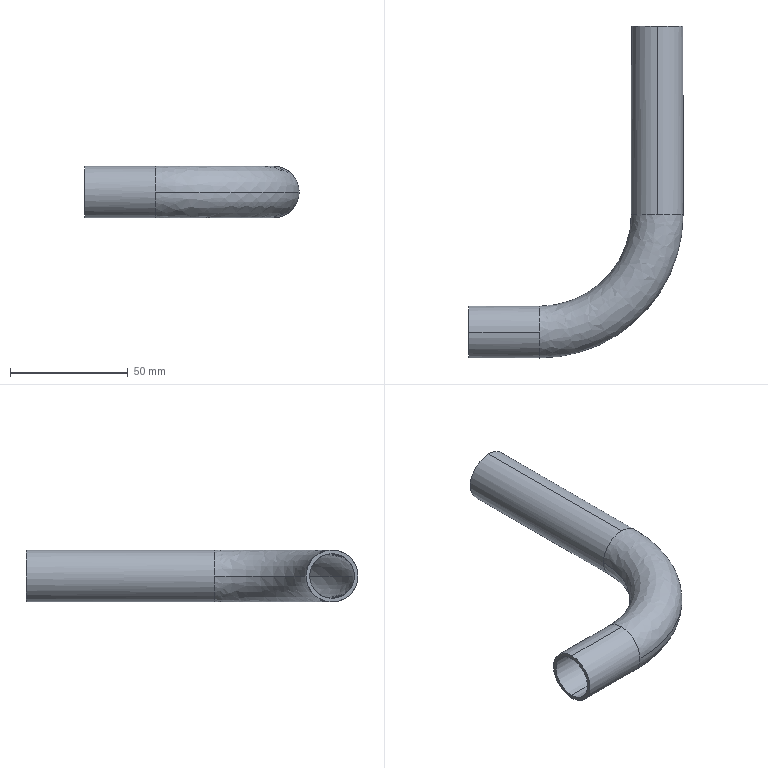Part | STEP file | copper tube 6_default_machined_ | 1 solid | 14 faces | box 91 x 141 x 22 mm | volume 18214 mm3 | cylinder 8 | spline 4 | plane 2 | commonest cylinder face diameters 19 x4 22 x4